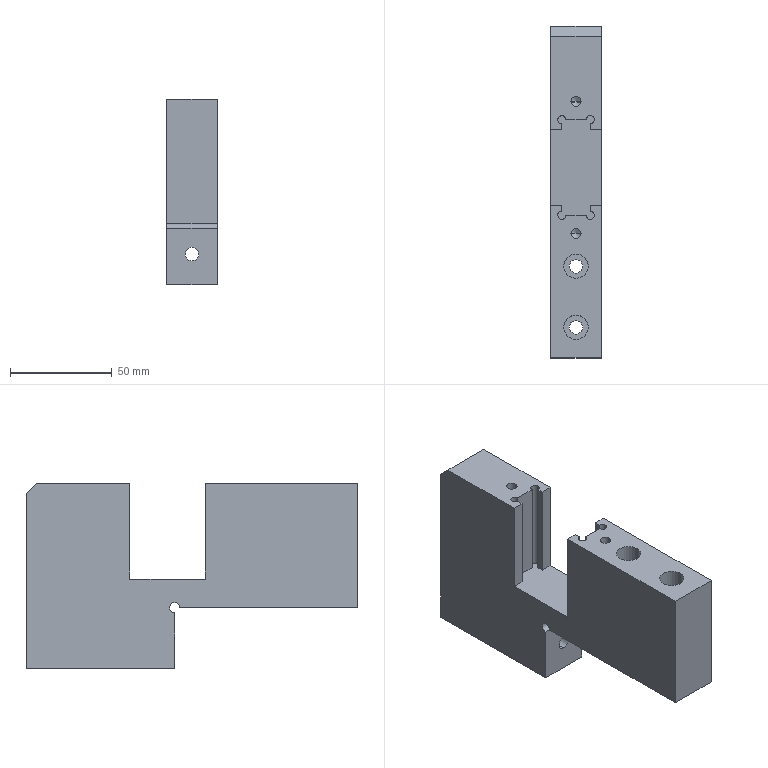Part | SolidWorks | features BaseBody 1 | 1 solid | 59 faces | box 25 x 163 x 91 mm | volume 230541 mm3 | cylinder 27 | plane 24 | cone 8 | commonest cylinder face diameters 4 x6 6.6 x6 12 x6 5 x5 4.2 x4